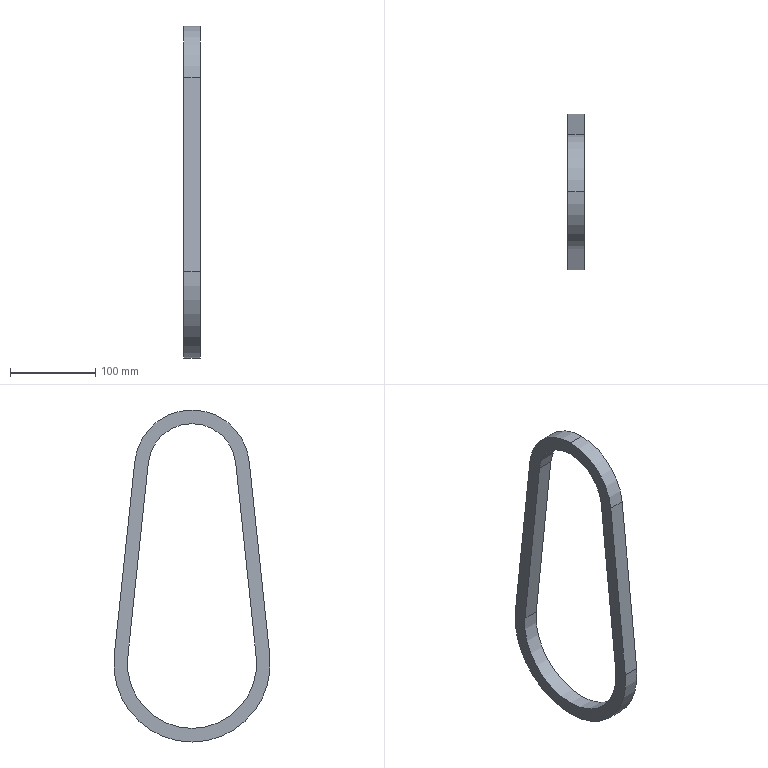Part | SolidWorks | features ExtruThin 1 | 1 solid | 12 faces | box 18.8 x 183.6 x 389.75 mm | volume 274842 mm3 | cylinder 6 | plane 6 | commonest cylinder face diameters 103.1 x2 135.1 x2 151.6 x1 183.6 x1
STEP:
#1=CARTESIAN_POINT('',(18.8,35.386,87.85));
#2=VERTEX_POINT('',#1);
#3=CARTESIAN_POINT('',(18.8,-15.878,133.974));
#4=VERTEX_POINT('',#3);
#5=CARTESIAN_POINT('',(18.8,-15.878,82.424));
#6=DIRECTION('',(1.,0.,0.));
#7=DIRECTION('',(0.,0.,-1.));
#8=AXIS2_PLACEMENT_3D('',#5,#6,#7);
#9=CIRCLE('',#8,51.55);
#10=EDGE_CURVE('',#2,#4,#9,.T.);
#11=ORIENTED_EDGE('',*,*,#10,.T.);
#12=CARTESIAN_POINT('',(0.,-15.878,133.974));
#13=VERTEX_POINT('',#12);
#14=CARTESIAN_POINT('',(18.8,-15.878,133.974));
#15=DIRECTION('',(-1.,0.,0.));
#16=VECTOR('',#15,1000.);
#17=LINE('',#14,#16);
#18=EDGE_CURVE('',#4,#13,#17,.T.);
#19=ORIENTED_EDGE('',*,*,#18,.T.);
#20=CARTESIAN_POINT('',(0.,35.386,87.85));
#21=VERTEX_POINT('',#20);
#22=CARTESIAN_POINT('',(0.,-15.878,82.424));
#23=DIRECTION('',(1.,0.,0.));
#24=DIRECTION('',(0.,0.,-1.));
#25=AXIS2_PLACEMENT_3D('',#22,#23,#24);
#26=CIRCLE('',#25,51.55);
#27=EDGE_CURVE('',#21,#13,#26,.T.);
#28=ORIENTED_EDGE('',*,*,#27,.F.);
#29=CARTESIAN_POINT('',(18.8,35.386,87.85));
#30=DIRECTION('',(-1.,0.,0.));
#31=VECTOR('',#30,1000.);
#32=LINE('',#29,#31);
#33=EDGE_CURVE('',#2,#21,#32,.T.);
#34=ORIENTED_EDGE('',*,*,#33,.F.);
#35=EDGE_LOOP('',(#11,#19,#28,#34));
#36=FACE_OUTER_BOUND('',#35,.T.);
#37=CARTESIAN_POINT('',(18.8,-15.878,82.424));
#38=DIRECTION('',(-1.,0.,0.));
#39=DIRECTION('',(0.,0.,1.));
#40=AXIS2_PLACEMENT_3D('',#37,#38,#39);
#41=CYLINDRICAL_SURFACE('',#40,51.55);
#42=ADVANCED_FACE('',(#36),#41,.F.);
#43=CARTESIAN_POINT('',(18.8,-15.878,149.974));
#44=VERTEX_POINT('',#43);
#45=CARTESIAN_POINT('',(18.8,-83.052,89.534));
#46=VERTEX_POINT('',#45);
#47=CARTESIAN_POINT('',(18.8,-15.878,82.424));
#48=DIRECTION('',(1.,0.,0.));
#49=DIRECTION('',(0.,0.,-1.));
#50=AXIS2_PLACEMENT_3D('',#47,#48,#49);
#51=CIRCLE('',#50,67.55);
#52=EDGE_CURVE('',#44,#46,#51,.T.);
#53=ORIENTED_EDGE('',*,*,#52,.F.);
#54=CARTESIAN_POINT('',(0.,-15.878,149.974));
#55=VERTEX_POINT('',#54);
#56=CARTESIAN_POINT('',(18.8,-15.878,149.974));
#57=DIRECTION('',(-1.,0.,0.));
#58=VECTOR('',#57,1000.);
#59=LINE('',#56,#58);
#60=EDGE_CURVE('',#44,#55,#59,.T.);
#61=ORIENTED_EDGE('',*,*,#60,.T.);
#62=CARTESIAN_POINT('',(0.,-83.052,89.534));
#63=VERTEX_POINT('',#62);
#64=CARTESIAN_POINT('',(0.,-15.878,82.424));
#65=DIRECTION('',(1.,0.,0.));
#66=DIRECTION('',(0.,0.,-1.));
#67=AXIS2_PLACEMENT_3D('',#64,#65,#66);
#68=CIRCLE('',#67,67.55);
#69=EDGE_CURVE('',#55,#63,#68,.T.);
#70=ORIENTED_EDGE('',*,*,#69,.T.);
#71=CARTESIAN_POINT('',(18.8,-83.052,89.534));
#72=DIRECTION('',(-1.,0.,0.));
#73=VECTOR('',#72,1000.);
#74=LINE('',#71,#73);
#75=EDGE_CURVE('',#46,#63,#74,.T.);
#76=ORIENTED_EDGE('',*,*,#75,.F.);
#77=EDGE_LOOP('',(#53,#61,#70,#76));
#78=FACE_OUTER_BOUND('',#77,.T.);
#79=CARTESIAN_POINT('',(18.8,-15.878,82.424));
#80=DIRECTION('',(-1.,0.,0.));
#81=DIRECTION('',(0.,0.,1.));
#82=AXIS2_PLACEMENT_3D('',#79,#80,#81);
#83=CYLINDRICAL_SURFACE('',#82,67.55);
#84=ADVANCED_FACE('',(#78),#83,.T.);
#85=CARTESIAN_POINT('',(18.8,51.297,89.534));
#86=VERTEX_POINT('',#85);
#87=CARTESIAN_POINT('',(18.8,-15.878,82.424));
#88=DIRECTION('',(1.,0.,0.));
#89=DIRECTION('',(0.,0.,-1.));
#90=AXIS2_PLACEMENT_3D('',#87,#88,#89);
#91=CIRCLE('',#90,67.55);
#92=EDGE_CURVE('',#86,#44,#91,.T.);
#93=ORIENTED_EDGE('',*,*,#92,.T.);
#94=ORIENTED_EDGE('',*,*,#52,.T.);
#95=CARTESIAN_POINT('',(18.8,-107.168,-138.314));
#96=VERTEX_POINT('',#95);
#97=CARTESIAN_POINT('',(18.8,-83.052,89.534));
#98=DIRECTION('',(0.,-0.1053,-0.9944));
#99=VECTOR('',#98,1000.);
#100=LINE('',#97,#99);
#101=EDGE_CURVE('',#46,#96,#100,.T.);
#102=ORIENTED_EDGE('',*,*,#101,.T.);
#103=CARTESIAN_POINT('',(18.8,75.413,-138.314));
#104=VERTEX_POINT('',#103);
#105=CARTESIAN_POINT('',(18.8,-15.878,-147.976));
#106=DIRECTION('',(1.,0.,0.));
#107=DIRECTION('',(0.,0.,-1.));
#108=AXIS2_PLACEMENT_3D('',#105,#106,#107);
#109=CIRCLE('',#108,91.8);
#110=EDGE_CURVE('',#96,#104,#109,.T.);
#111=ORIENTED_EDGE('',*,*,#110,.T.);
#112=CARTESIAN_POINT('',(18.8,51.297,89.534));
#113=DIRECTION('',(0.,-0.1053,0.9944));
#114=VECTOR('',#113,1000.);
#115=LINE('',#112,#114);
#116=EDGE_CURVE('',#104,#86,#115,.T.);
#117=ORIENTED_EDGE('',*,*,#116,.T.);
#118=EDGE_LOOP('',(#93,#94,#102,#111,#117));
#119=FACE_OUTER_BOUND('',#118,.T.);
#120=CARTESIAN_POINT('',(18.8,-67.141,87.85));
#121=VERTEX_POINT('',#120);
#122=CARTESIAN_POINT('',(18.8,-91.257,-139.998));
#123=VERTEX_POINT('',#122);
#124=CARTESIAN_POINT('',(18.8,-67.141,87.85));
#125=DIRECTION('',(0.,-0.1053,-0.9944));
#126=VECTOR('',#125,1000.);
#127=LINE('',#124,#126);
#128=EDGE_CURVE('',#121,#123,#127,.T.);
#129=ORIENTED_EDGE('',*,*,#128,.F.);
#130=CARTESIAN_POINT('',(18.8,-15.878,82.424));
#131=DIRECTION('',(1.,0.,0.));
#132=DIRECTION('',(0.,0.,-1.));
#133=AXIS2_PLACEMENT_3D('',#130,#131,#132);
#134=CIRCLE('',#133,51.55);
#135=EDGE_CURVE('',#4,#121,#134,.T.);
#136=ORIENTED_EDGE('',*,*,#135,.F.);
#137=ORIENTED_EDGE('',*,*,#10,.F.);
#138=CARTESIAN_POINT('',(18.8,59.501,-139.998));
#139=VERTEX_POINT('',#138);
#140=CARTESIAN_POINT('',(18.8,35.386,87.85));
#141=DIRECTION('',(0.,-0.1053,0.9944));
#142=VECTOR('',#141,1000.);
#143=LINE('',#140,#142);
#144=EDGE_CURVE('',#139,#2,#143,.T.);
#145=ORIENTED_EDGE('',*,*,#144,.F.);
#146=CARTESIAN_POINT('',(18.8,-15.878,-147.976));
#147=DIRECTION('',(1.,0.,0.));
#148=DIRECTION('',(0.,0.,-1.));
#149=AXIS2_PLACEMENT_3D('',#146,#147,#148);
#150=CIRCLE('',#149,75.8);
#151=EDGE_CURVE('',#123,#139,#150,.T.);
#152=ORIENTED_EDGE('',*,*,#151,.F.);
#153=EDGE_LOOP('',(#129,#136,#137,#145,#152));
#154=FACE_BOUND('',#153,.T.);
#155=CARTESIAN_POINT('',(18.8,-15.878,82.424));
#156=DIRECTION('',(1.,0.,0.));
#157=DIRECTION('',(0.,0.,-1.));
#158=AXIS2_PLACEMENT_3D('',#155,#156,#157);
#159=PLANE('',#158);
#160=ADVANCED_FACE('',(#119,#154),#159,.T.);
#161=CARTESIAN_POINT('',(0.,51.297,89.534));
#162=VERTEX_POINT('',#161);
#163=CARTESIAN_POINT('',(0.,-15.878,82.424));
#164=DIRECTION('',(1.,0.,0.));
#165=DIRECTION('',(0.,0.,-1.));
#166=AXIS2_PLACEMENT_3D('',#163,#164,#165);
#167=CIRCLE('',#166,67.55);
#168=EDGE_CURVE('',#162,#55,#167,.T.);
#169=ORIENTED_EDGE('',*,*,#168,.F.);
#170=CARTESIAN_POINT('',(0.,75.413,-138.314));
#171=VERTEX_POINT('',#170);
#172=CARTESIAN_POINT('',(0.,51.297,89.534));
#173=DIRECTION('',(0.,-0.1053,0.9944));
#174=VECTOR('',#173,1000.);
#175=LINE('',#172,#174);
#176=EDGE_CURVE('',#171,#162,#175,.T.);
#177=ORIENTED_EDGE('',*,*,#176,.F.);
#178=CARTESIAN_POINT('',(0.,-107.168,-138.314));
#179=VERTEX_POINT('',#178);
#180=CARTESIAN_POINT('',(0.,-15.878,-147.976));
#181=DIRECTION('',(1.,0.,0.));
#182=DIRECTION('',(0.,0.,-1.));
#183=AXIS2_PLACEMENT_3D('',#180,#181,#182);
#184=CIRCLE('',#183,91.8);
#185=EDGE_CURVE('',#179,#171,#184,.T.);
#186=ORIENTED_EDGE('',*,*,#185,.F.);
#187=CARTESIAN_POINT('',(0.,-83.052,89.534));
#188=DIRECTION('',(0.,-0.1053,-0.9944));
#189=VECTOR('',#188,1000.);
#190=LINE('',#187,#189);
#191=EDGE_CURVE('',#63,#179,#190,.T.);
#192=ORIENTED_EDGE('',*,*,#191,.F.);
#193=ORIENTED_EDGE('',*,*,#69,.F.);
#194=EDGE_LOOP('',(#169,#177,#186,#192,#193));
#195=FACE_OUTER_BOUND('',#194,.T.);
#196=ORIENTED_EDGE('',*,*,#27,.T.);
#197=CARTESIAN_POINT('',(0.,-67.141,87.85));
#198=VERTEX_POINT('',#197);
#199=CARTESIAN_POINT('',(0.,-15.878,82.424));
#200=DIRECTION('',(1.,0.,0.));
#201=DIRECTION('',(0.,0.,-1.));
#202=AXIS2_PLACEMENT_3D('',#199,#200,#201);
#203=CIRCLE('',#202,51.55);
#204=EDGE_CURVE('',#13,#198,#203,.T.);
#205=ORIENTED_EDGE('',*,*,#204,.T.);
#206=CARTESIAN_POINT('',(0.,-91.257,-139.998));
#207=VERTEX_POINT('',#206);
#208=CARTESIAN_POINT('',(0.,-67.141,87.85));
#209=DIRECTION('',(0.,-0.1053,-0.9944));
#210=VECTOR('',#209,1000.);
#211=LINE('',#208,#210);
#212=EDGE_CURVE('',#198,#207,#211,.T.);
#213=ORIENTED_EDGE('',*,*,#212,.T.);
#214=CARTESIAN_POINT('',(0.,59.501,-139.998));
#215=VERTEX_POINT('',#214);
#216=CARTESIAN_POINT('',(0.,-15.878,-147.976));
#217=DIRECTION('',(1.,0.,0.));
#218=DIRECTION('',(0.,0.,-1.));
#219=AXIS2_PLACEMENT_3D('',#216,#217,#218);
#220=CIRCLE('',#219,75.8);
#221=EDGE_CURVE('',#207,#215,#220,.T.);
#222=ORIENTED_EDGE('',*,*,#221,.T.);
#223=CARTESIAN_POINT('',(0.,35.386,87.85));
#224=DIRECTION('',(0.,-0.1053,0.9944));
#225=VECTOR('',#224,1000.);
#226=LINE('',#223,#225);
#227=EDGE_CURVE('',#215,#21,#226,.T.);
#228=ORIENTED_EDGE('',*,*,#227,.T.);
#229=EDGE_LOOP('',(#196,#205,#213,#222,#228));
#230=FACE_BOUND('',#229,.T.);
#231=CARTESIAN_POINT('',(0.,-15.878,82.424));
#232=DIRECTION('',(1.,0.,0.));
#233=DIRECTION('',(0.,0.,-1.));
#234=AXIS2_PLACEMENT_3D('',#231,#232,#233);
#235=PLANE('',#234);
#236=ADVANCED_FACE('',(#195,#230),#235,.F.);
#237=ORIENTED_EDGE('',*,*,#60,.F.);
#238=ORIENTED_EDGE('',*,*,#92,.F.);
#239=CARTESIAN_POINT('',(18.8,51.297,89.534));
#240=DIRECTION('',(-1.,0.,0.));
#241=VECTOR('',#240,1000.);
#242=LINE('',#239,#241);
#243=EDGE_CURVE('',#86,#162,#242,.T.);
#244=ORIENTED_EDGE('',*,*,#243,.T.);
#245=ORIENTED_EDGE('',*,*,#168,.T.);
#246=EDGE_LOOP('',(#237,#238,#244,#245));
#247=FACE_OUTER_BOUND('',#246,.T.);
#248=CARTESIAN_POINT('',(18.8,-15.878,82.424));
#249=DIRECTION('',(-1.,0.,0.));
#250=DIRECTION('',(0.,0.,1.));
#251=AXIS2_PLACEMENT_3D('',#248,#249,#250);
#252=CYLINDRICAL_SURFACE('',#251,67.55);
#253=ADVANCED_FACE('',(#247),#252,.T.);
#254=ORIENTED_EDGE('',*,*,#191,.T.);
#255=CARTESIAN_POINT('',(18.8,-107.168,-138.314));
#256=DIRECTION('',(-1.,0.,0.));
#257=VECTOR('',#256,1000.);
#258=LINE('',#255,#257);
#259=EDGE_CURVE('',#96,#179,#258,.T.);
#260=ORIENTED_EDGE('',*,*,#259,.F.);
#261=ORIENTED_EDGE('',*,*,#101,.F.);
#262=ORIENTED_EDGE('',*,*,#75,.T.);
#263=EDGE_LOOP('',(#254,#260,#261,#262));
#264=FACE_OUTER_BOUND('',#263,.T.);
#265=CARTESIAN_POINT('',(18.8,-83.052,89.534));
#266=DIRECTION('',(0.,0.9944,-0.1053));
#267=DIRECTION('',(0.,0.1053,0.9944));
#268=AXIS2_PLACEMENT_3D('',#265,#266,#267);
#269=PLANE('',#268);
#270=ADVANCED_FACE('',(#264),#269,.F.);
#271=ORIENTED_EDGE('',*,*,#185,.T.);
#272=CARTESIAN_POINT('',(18.8,75.413,-138.314));
#273=DIRECTION('',(-1.,0.,0.));
#274=VECTOR('',#273,1000.);
#275=LINE('',#272,#274);
#276=EDGE_CURVE('',#104,#171,#275,.T.);
#277=ORIENTED_EDGE('',*,*,#276,.F.);
#278=ORIENTED_EDGE('',*,*,#110,.F.);
#279=ORIENTED_EDGE('',*,*,#259,.T.);
#280=EDGE_LOOP('',(#271,#277,#278,#279));
#281=FACE_OUTER_BOUND('',#280,.T.);
#282=CARTESIAN_POINT('',(18.8,-15.878,-147.976));
#283=DIRECTION('',(-1.,0.,0.));
#284=DIRECTION('',(0.,0.,1.));
#285=AXIS2_PLACEMENT_3D('',#282,#283,#284);
#286=CYLINDRICAL_SURFACE('',#285,91.8);
#287=ADVANCED_FACE('',(#281),#286,.T.);
#288=ORIENTED_EDGE('',*,*,#176,.T.);
#289=ORIENTED_EDGE('',*,*,#243,.F.);
#290=ORIENTED_EDGE('',*,*,#116,.F.);
#291=ORIENTED_EDGE('',*,*,#276,.T.);
#292=EDGE_LOOP('',(#288,#289,#290,#291));
#293=FACE_OUTER_BOUND('',#292,.T.);
#294=CARTESIAN_POINT('',(18.8,51.297,89.534));
#295=DIRECTION('',(0.,-0.9944,-0.1053));
#296=DIRECTION('',(0.,0.1053,-0.9944));
#297=AXIS2_PLACEMENT_3D('',#294,#295,#296);
#298=PLANE('',#297);
#299=ADVANCED_FACE('',(#293),#298,.F.);
#300=ORIENTED_EDGE('',*,*,#18,.F.);
#301=ORIENTED_EDGE('',*,*,#135,.T.);
#302=CARTESIAN_POINT('',(18.8,-67.141,87.85));
#303=DIRECTION('',(-1.,0.,0.));
#304=VECTOR('',#303,1000.);
#305=LINE('',#302,#304);
#306=EDGE_CURVE('',#121,#198,#305,.T.);
#307=ORIENTED_EDGE('',*,*,#306,.T.);
#308=ORIENTED_EDGE('',*,*,#204,.F.);
#309=EDGE_LOOP('',(#300,#301,#307,#308));
#310=FACE_OUTER_BOUND('',#309,.T.);
#311=CARTESIAN_POINT('',(18.8,-15.878,82.424));
#312=DIRECTION('',(-1.,0.,0.));
#313=DIRECTION('',(0.,0.,1.));
#314=AXIS2_PLACEMENT_3D('',#311,#312,#313);
#315=CYLINDRICAL_SURFACE('',#314,51.55);
#316=ADVANCED_FACE('',(#310),#315,.F.);
#317=ORIENTED_EDGE('',*,*,#212,.F.);
#318=ORIENTED_EDGE('',*,*,#306,.F.);
#319=ORIENTED_EDGE('',*,*,#128,.T.);
#320=CARTESIAN_POINT('',(18.8,-91.257,-139.998));
#321=DIRECTION('',(-1.,0.,0.));
#322=VECTOR('',#321,1000.);
#323=LINE('',#320,#322);
#324=EDGE_CURVE('',#123,#207,#323,.T.);
#325=ORIENTED_EDGE('',*,*,#324,.T.);
#326=EDGE_LOOP('',(#317,#318,#319,#325));
#327=FACE_OUTER_BOUND('',#326,.T.);
#328=CARTESIAN_POINT('',(18.8,-67.141,87.85));
#329=DIRECTION('',(0.,0.9944,-0.1053));
#330=DIRECTION('',(0.,0.1053,0.9944));
#331=AXIS2_PLACEMENT_3D('',#328,#329,#330);
#332=PLANE('',#331);
#333=ADVANCED_FACE('',(#327),#332,.T.);
#334=ORIENTED_EDGE('',*,*,#221,.F.);
#335=ORIENTED_EDGE('',*,*,#324,.F.);
#336=ORIENTED_EDGE('',*,*,#151,.T.);
#337=CARTESIAN_POINT('',(18.8,59.501,-139.998));
#338=DIRECTION('',(-1.,0.,0.));
#339=VECTOR('',#338,1000.);
#340=LINE('',#337,#339);
#341=EDGE_CURVE('',#139,#215,#340,.T.);
#342=ORIENTED_EDGE('',*,*,#341,.T.);
#343=EDGE_LOOP('',(#334,#335,#336,#342));
#344=FACE_OUTER_BOUND('',#343,.T.);
#345=CARTESIAN_POINT('',(18.8,-15.878,-147.976));
#346=DIRECTION('',(-1.,0.,0.));
#347=DIRECTION('',(0.,0.,1.));
#348=AXIS2_PLACEMENT_3D('',#345,#346,#347);
#349=CYLINDRICAL_SURFACE('',#348,75.8);
#350=ADVANCED_FACE('',(#344),#349,.F.);
#351=ORIENTED_EDGE('',*,*,#227,.F.);
#352=ORIENTED_EDGE('',*,*,#341,.F.);
#353=ORIENTED_EDGE('',*,*,#144,.T.);
#354=ORIENTED_EDGE('',*,*,#33,.T.);
#355=EDGE_LOOP('',(#351,#352,#353,#354));
#356=FACE_OUTER_BOUND('',#355,.T.);
#357=CARTESIAN_POINT('',(18.8,35.386,87.85));
#358=DIRECTION('',(0.,-0.9944,-0.1053));
#359=DIRECTION('',(0.,0.1053,-0.9944));
#360=AXIS2_PLACEMENT_3D('',#357,#358,#359);
#361=PLANE('',#360);
#362=ADVANCED_FACE('',(#356),#361,.T.);
#363=CLOSED_SHELL('',(#42,#84,#160,#236,#253,#270,#287,#299,#316,#333,#350,#362));
#364=MANIFOLD_SOLID_BREP('',#363);
#365=CARTESIAN_POINT('',(0.,0.,0.));
#366=DIRECTION('',(0.,0.,1.));
#367=DIRECTION('',(1.,0.,0.));
#368=AXIS2_PLACEMENT_3D('',#365,#366,#367);
#369=(LENGTH_UNIT()NAMED_UNIT(*)SI_UNIT(.MILLI.,.METRE.));
#370=UNCERTAINTY_MEASURE_WITH_UNIT(LENGTH_MEASURE(0.00001),#369,'','');
#371=(NAMED_UNIT(*)PLANE_ANGLE_UNIT()SI_UNIT($,.RADIAN.));
#372=(NAMED_UNIT(*)SI_UNIT($,.STERADIAN.)SOLID_ANGLE_UNIT());
#373=(GEOMETRIC_REPRESENTATION_CONTEXT(3)GLOBAL_UNCERTAINTY_ASSIGNED_CONTEXT((#370))GLOBAL_UNIT_ASSIGNED_CONTEXT((#369,#371,#372))REPRESENTATION_CONTEXT('',''));
#374=ADVANCED_BREP_SHAPE_REPRESENTATION('',(#364,#368),#373);